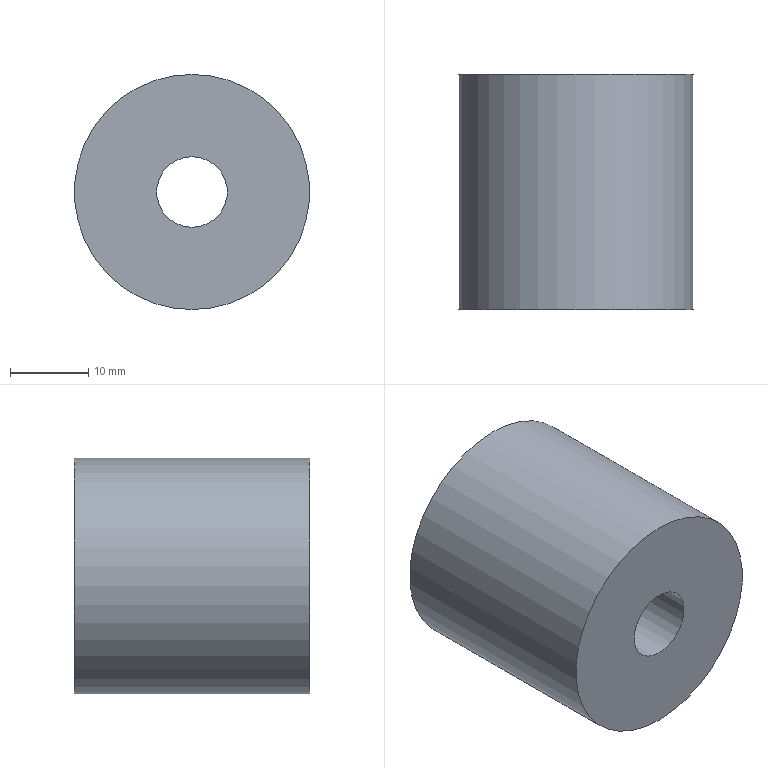Part | NX | features solid 2 | 1 solid | 6 faces | box 30 x 30 x 30 mm | volume 17491 mm3 | cylinder 3 | plane 3 | commonest cylinder face diameters 9 x1 14 x1 30 x1
STEP:
#1=CARTESIAN_POINT('',(-1045.,-585.,-370.));
#2=VERTEX_POINT('',#1);
#3=CARTESIAN_POINT('',(-1045.,-585.,-355.));
#4=DIRECTION('',(0.,1.,0.));
#5=DIRECTION('',(0.,0.,-1.));
#6=AXIS2_PLACEMENT_3D('',#3,#4,#5);
#7=CIRCLE('',#6,15.);
#8=EDGE_CURVE('',#2,#2,#7,.T.);
#9=ORIENTED_EDGE('',*,*,#8,.F.);
#10=EDGE_LOOP('',(#9));
#11=FACE_BOUND('',#10,.T.);
#12=CARTESIAN_POINT('',(-1045.,-615.,-370.));
#13=VERTEX_POINT('',#12);
#14=CARTESIAN_POINT('',(-1045.,-615.,-355.));
#15=DIRECTION('',(0.,1.,0.));
#16=DIRECTION('',(0.,0.,-1.));
#17=AXIS2_PLACEMENT_3D('',#14,#15,#16);
#18=CIRCLE('',#17,15.);
#19=EDGE_CURVE('',#13,#13,#18,.T.);
#20=ORIENTED_EDGE('',*,*,#19,.T.);
#21=EDGE_LOOP('',(#20));
#22=FACE_BOUND('',#21,.T.);
#23=CARTESIAN_POINT('',(-1045.,-585.,-355.));
#24=DIRECTION('',(0.,-1.,0.));
#25=DIRECTION('',(0.,0.,-1.));
#26=AXIS2_PLACEMENT_3D('',#23,#24,#25);
#27=CYLINDRICAL_SURFACE('',#26,15.);
#28=ADVANCED_FACE('',(#11,#22),#27,.T.);
#29=CARTESIAN_POINT('',(-1045.,-585.,-362.));
#30=VERTEX_POINT('',#29);
#31=CARTESIAN_POINT('',(-1045.,-585.,-355.));
#32=DIRECTION('',(0.,1.,0.));
#33=DIRECTION('',(0.,0.,-1.));
#34=AXIS2_PLACEMENT_3D('',#31,#32,#33);
#35=CIRCLE('',#34,7.);
#36=EDGE_CURVE('',#30,#30,#35,.T.);
#37=ORIENTED_EDGE('',*,*,#36,.F.);
#38=EDGE_LOOP('',(#37));
#39=FACE_BOUND('',#38,.T.);
#40=ORIENTED_EDGE('',*,*,#8,.T.);
#41=EDGE_LOOP('',(#40));
#42=FACE_BOUND('',#41,.T.);
#43=CARTESIAN_POINT('',(-1045.,-585.,-355.));
#44=DIRECTION('',(0.,-1.,0.));
#45=DIRECTION('',(0.,0.,-1.));
#46=AXIS2_PLACEMENT_3D('',#43,#44,#45);
#47=PLANE('',#46);
#48=ADVANCED_FACE('',(#39,#42),#47,.F.);
#49=CARTESIAN_POINT('',(-1045.,-615.,-359.5));
#50=VERTEX_POINT('',#49);
#51=CARTESIAN_POINT('',(-1045.,-615.,-355.));
#52=DIRECTION('',(0.,1.,0.));
#53=DIRECTION('',(0.,0.,-1.));
#54=AXIS2_PLACEMENT_3D('',#51,#52,#53);
#55=CIRCLE('',#54,4.5);
#56=EDGE_CURVE('',#50,#50,#55,.T.);
#57=ORIENTED_EDGE('',*,*,#56,.T.);
#58=EDGE_LOOP('',(#57));
#59=FACE_BOUND('',#58,.T.);
#60=ORIENTED_EDGE('',*,*,#19,.F.);
#61=EDGE_LOOP('',(#60));
#62=FACE_BOUND('',#61,.T.);
#63=CARTESIAN_POINT('',(-1045.,-615.,-355.));
#64=DIRECTION('',(0.,-1.,0.));
#65=DIRECTION('',(0.,0.,-1.));
#66=AXIS2_PLACEMENT_3D('',#63,#64,#65);
#67=PLANE('',#66);
#68=ADVANCED_FACE('',(#59,#62),#67,.T.);
#69=ORIENTED_EDGE('',*,*,#56,.F.);
#70=EDGE_LOOP('',(#69));
#71=FACE_BOUND('',#70,.T.);
#72=CARTESIAN_POINT('',(-1045.,-605.,-359.5));
#73=VERTEX_POINT('',#72);
#74=CARTESIAN_POINT('',(-1045.,-605.,-355.));
#75=DIRECTION('',(0.,1.,0.));
#76=DIRECTION('',(0.,0.,-1.));
#77=AXIS2_PLACEMENT_3D('',#74,#75,#76);
#78=CIRCLE('',#77,4.5);
#79=EDGE_CURVE('',#73,#73,#78,.T.);
#80=ORIENTED_EDGE('',*,*,#79,.T.);
#81=EDGE_LOOP('',(#80));
#82=FACE_BOUND('',#81,.T.);
#83=CARTESIAN_POINT('',(-1045.,-635.,-355.));
#84=DIRECTION('',(0.,-1.,0.));
#85=DIRECTION('',(0.,0.,-1.));
#86=AXIS2_PLACEMENT_3D('',#83,#84,#85);
#87=CYLINDRICAL_SURFACE('',#86,4.5);
#88=ADVANCED_FACE('',(#71,#82),#87,.F.);
#89=ORIENTED_EDGE('',*,*,#79,.F.);
#90=EDGE_LOOP('',(#89));
#91=FACE_BOUND('',#90,.T.);
#92=CARTESIAN_POINT('',(-1045.,-605.,-362.));
#93=VERTEX_POINT('',#92);
#94=CARTESIAN_POINT('',(-1045.,-605.,-355.));
#95=DIRECTION('',(0.,1.,0.));
#96=DIRECTION('',(0.,0.,-1.));
#97=AXIS2_PLACEMENT_3D('',#94,#95,#96);
#98=CIRCLE('',#97,7.);
#99=EDGE_CURVE('',#93,#93,#98,.T.);
#100=ORIENTED_EDGE('',*,*,#99,.T.);
#101=EDGE_LOOP('',(#100));
#102=FACE_BOUND('',#101,.T.);
#103=CARTESIAN_POINT('',(-1045.,-605.,-355.));
#104=DIRECTION('',(0.,-1.,0.));
#105=DIRECTION('',(0.,0.,-1.));
#106=AXIS2_PLACEMENT_3D('',#103,#104,#105);
#107=PLANE('',#106);
#108=ADVANCED_FACE('',(#91,#102),#107,.F.);
#109=ORIENTED_EDGE('',*,*,#99,.F.);
#110=EDGE_LOOP('',(#109));
#111=FACE_BOUND('',#110,.T.);
#112=ORIENTED_EDGE('',*,*,#36,.T.);
#113=EDGE_LOOP('',(#112));
#114=FACE_BOUND('',#113,.T.);
#115=CARTESIAN_POINT('',(-1045.,-585.,-355.));
#116=DIRECTION('',(0.,-1.,0.));
#117=DIRECTION('',(0.,0.,-1.));
#118=AXIS2_PLACEMENT_3D('',#115,#116,#117);
#119=CYLINDRICAL_SURFACE('',#118,7.);
#120=ADVANCED_FACE('',(#111,#114),#119,.F.);
#121=CLOSED_SHELL('',(#28,#48,#68,#88,#108,#120));
#122=MANIFOLD_SOLID_BREP('',#121);
#123=(LENGTH_UNIT()NAMED_UNIT(*)SI_UNIT(.MILLI.,.METRE.));
#124=UNCERTAINTY_MEASURE_WITH_UNIT(LENGTH_MEASURE(0.00001),#123,'','');
#125=(NAMED_UNIT(*)PLANE_ANGLE_UNIT()SI_UNIT($,.RADIAN.));
#126=(NAMED_UNIT(*)SI_UNIT($,.STERADIAN.)SOLID_ANGLE_UNIT());
#127=(GEOMETRIC_REPRESENTATION_CONTEXT(3)GLOBAL_UNCERTAINTY_ASSIGNED_CONTEXT((#124))GLOBAL_UNIT_ASSIGNED_CONTEXT((#123,#125,#126))REPRESENTATION_CONTEXT('',''));
#128=ADVANCED_BREP_SHAPE_REPRESENTATION('',(#122),#127);